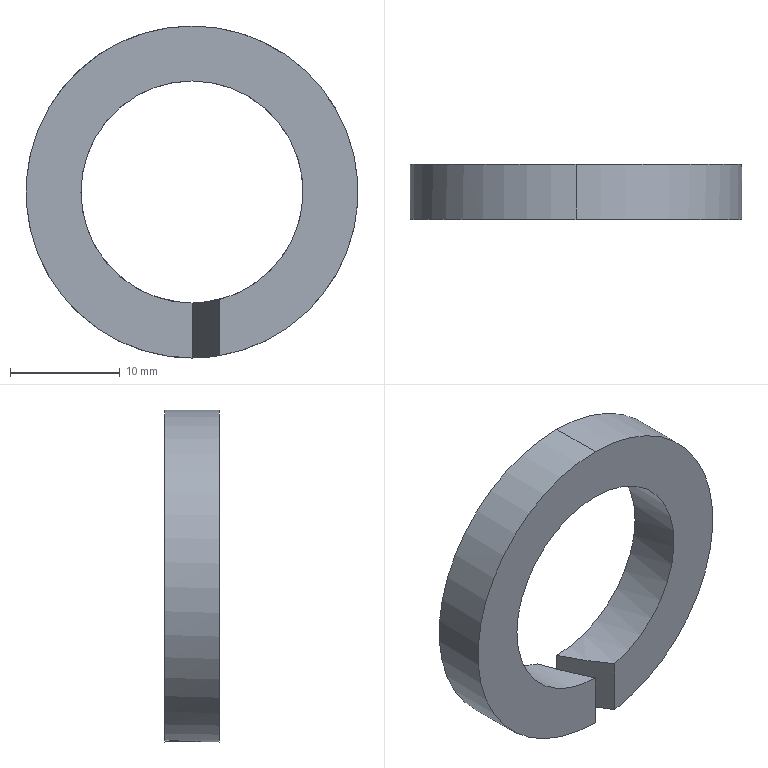Part | SolidWorks | features BaseBody 1 | 1 solid | 8 faces | box 30.2 x 5 x 30.2 mm | volume 1916 mm3 | cylinder 4 | plane 4 | commonest cylinder face diameters 20.2 x2 30.2 x2
STEP:
#1=CARTESIAN_POINT('',(2.5,0.,-9.786));
#2=VERTEX_POINT('',#1);
#3=CARTESIAN_POINT('',(0.,0.,10.1));
#4=VERTEX_POINT('',#3);
#5=CARTESIAN_POINT('',(0.,0.,0.));
#6=DIRECTION('',(0.,-1.,0.));
#7=DIRECTION('',(0.,0.,1.));
#8=AXIS2_PLACEMENT_3D('',#5,#6,#7);
#9=CIRCLE('',#8,10.1);
#10=EDGE_CURVE('',#2,#4,#9,.T.);
#11=ORIENTED_EDGE('',*,*,#10,.T.);
#12=CARTESIAN_POINT('',(0.,5.,10.1));
#13=VERTEX_POINT('',#12);
#14=CARTESIAN_POINT('',(0.,0.,10.1));
#15=DIRECTION('',(0.,1.,0.));
#16=VECTOR('',#15,1000.);
#17=LINE('',#14,#16);
#18=EDGE_CURVE('',#4,#13,#17,.T.);
#19=ORIENTED_EDGE('',*,*,#18,.T.);
#20=CARTESIAN_POINT('',(0.,5.,-10.1));
#21=VERTEX_POINT('',#20);
#22=CARTESIAN_POINT('',(0.,5.,0.));
#23=DIRECTION('',(0.,-1.,0.));
#24=DIRECTION('',(0.,0.,1.));
#25=AXIS2_PLACEMENT_3D('',#22,#23,#24);
#26=CIRCLE('',#25,10.1);
#27=EDGE_CURVE('',#21,#13,#26,.T.);
#28=ORIENTED_EDGE('',*,*,#27,.F.);
#29=CARTESIAN_POINT('',(2.5,0.,-9.786));
#30=CARTESIAN_POINT('',(1.682,1.636,-9.995));
#31=CARTESIAN_POINT('',(0.8443,3.311,-10.1));
#32=CARTESIAN_POINT('',(0.,5.,-10.1));
#33=(BOUNDED_CURVE()B_SPLINE_CURVE(3,(#29,#30,#31,#32),.UNSPECIFIED.,.F.,.F.)B_SPLINE_CURVE_WITH_KNOTS((4,4),(4.462,4.712),.UNSPECIFIED.)CURVE()GEOMETRIC_REPRESENTATION_ITEM()RATIONAL_B_SPLINE_CURVE((1.,0.9948,0.9948,1.))REPRESENTATION_ITEM(''));
#34=EDGE_CURVE('',#2,#21,#33,.T.);
#35=ORIENTED_EDGE('',*,*,#34,.F.);
#36=EDGE_LOOP('',(#11,#19,#28,#35));
#37=FACE_OUTER_BOUND('',#36,.T.);
#38=CARTESIAN_POINT('',(0.,0.,0.));
#39=DIRECTION('',(0.,1.,0.));
#40=DIRECTION('',(0.,0.,1.));
#41=AXIS2_PLACEMENT_3D('',#38,#39,#40);
#42=CYLINDRICAL_SURFACE('',#41,10.1);
#43=ADVANCED_FACE('',(#37),#42,.F.);
#44=CARTESIAN_POINT('',(0.,0.,-15.1));
#45=VERTEX_POINT('',#44);
#46=CARTESIAN_POINT('',(0.,0.,15.1));
#47=VERTEX_POINT('',#46);
#48=CARTESIAN_POINT('',(0.,0.,0.));
#49=DIRECTION('',(0.,1.,0.));
#50=DIRECTION('',(0.,0.,1.));
#51=AXIS2_PLACEMENT_3D('',#48,#49,#50);
#52=CIRCLE('',#51,15.1);
#53=EDGE_CURVE('',#45,#47,#52,.T.);
#54=ORIENTED_EDGE('',*,*,#53,.T.);
#55=CARTESIAN_POINT('',(0.,5.,15.1));
#56=VERTEX_POINT('',#55);
#57=CARTESIAN_POINT('',(0.,0.,15.1));
#58=DIRECTION('',(0.,1.,0.));
#59=VECTOR('',#58,1000.);
#60=LINE('',#57,#59);
#61=EDGE_CURVE('',#47,#56,#60,.T.);
#62=ORIENTED_EDGE('',*,*,#61,.T.);
#63=CARTESIAN_POINT('',(-2.5,5.,-14.892));
#64=VERTEX_POINT('',#63);
#65=CARTESIAN_POINT('',(0.,5.,0.));
#66=DIRECTION('',(0.,-1.,0.));
#67=DIRECTION('',(0.,0.,1.));
#68=AXIS2_PLACEMENT_3D('',#65,#66,#67);
#69=CIRCLE('',#68,15.1);
#70=EDGE_CURVE('',#56,#64,#69,.T.);
#71=ORIENTED_EDGE('',*,*,#70,.T.);
#72=CARTESIAN_POINT('',(-2.5,5.,-14.892));
#73=CARTESIAN_POINT('',(-1.673,3.347,-15.03));
#74=CARTESIAN_POINT('',(-0.8382,1.676,-15.1));
#75=CARTESIAN_POINT('',(0.,0.,-15.1));
#76=(BOUNDED_CURVE()B_SPLINE_CURVE(3,(#72,#73,#74,#75),.UNSPECIFIED.,.F.,.F.)B_SPLINE_CURVE_WITH_KNOTS((4,4),(1.404,1.571),.UNSPECIFIED.)CURVE()GEOMETRIC_REPRESENTATION_ITEM()RATIONAL_B_SPLINE_CURVE((1.,0.9977,0.9977,1.))REPRESENTATION_ITEM(''));
#77=EDGE_CURVE('',#64,#45,#76,.T.);
#78=ORIENTED_EDGE('',*,*,#77,.T.);
#79=EDGE_LOOP('',(#54,#62,#71,#78));
#80=FACE_OUTER_BOUND('',#79,.T.);
#81=CARTESIAN_POINT('',(0.,0.,0.));
#82=DIRECTION('',(0.,1.,0.));
#83=DIRECTION('',(0.,0.,1.));
#84=AXIS2_PLACEMENT_3D('',#81,#82,#83);
#85=CYLINDRICAL_SURFACE('',#84,15.1);
#86=ADVANCED_FACE('',(#80),#85,.T.);
#87=CARTESIAN_POINT('',(2.5,0.,-14.892));
#88=VERTEX_POINT('',#87);
#89=CARTESIAN_POINT('',(2.5,0.,0.));
#90=DIRECTION('',(0.,0.,1.));
#91=VECTOR('',#90,1000.);
#92=LINE('',#89,#91);
#93=EDGE_CURVE('',#88,#2,#92,.T.);
#94=ORIENTED_EDGE('',*,*,#93,.F.);
#95=CARTESIAN_POINT('',(0.,0.,0.));
#96=DIRECTION('',(0.,1.,0.));
#97=DIRECTION('',(0.,0.,1.));
#98=AXIS2_PLACEMENT_3D('',#95,#96,#97);
#99=CIRCLE('',#98,15.1);
#100=EDGE_CURVE('',#47,#88,#99,.T.);
#101=ORIENTED_EDGE('',*,*,#100,.F.);
#102=ORIENTED_EDGE('',*,*,#53,.F.);
#103=CARTESIAN_POINT('',(0.,0.,-10.1));
#104=VERTEX_POINT('',#103);
#105=CARTESIAN_POINT('',(0.,0.,0.));
#106=DIRECTION('',(0.,0.,-1.));
#107=VECTOR('',#106,1000.);
#108=LINE('',#105,#107);
#109=EDGE_CURVE('',#104,#45,#108,.T.);
#110=ORIENTED_EDGE('',*,*,#109,.F.);
#111=CARTESIAN_POINT('',(0.,0.,0.));
#112=DIRECTION('',(0.,-1.,0.));
#113=DIRECTION('',(0.,0.,1.));
#114=AXIS2_PLACEMENT_3D('',#111,#112,#113);
#115=CIRCLE('',#114,10.1);
#116=EDGE_CURVE('',#4,#104,#115,.T.);
#117=ORIENTED_EDGE('',*,*,#116,.F.);
#118=ORIENTED_EDGE('',*,*,#10,.F.);
#119=EDGE_LOOP('',(#94,#101,#102,#110,#117,#118));
#120=FACE_OUTER_BOUND('',#119,.T.);
#121=CARTESIAN_POINT('',(0.,0.,0.));
#122=DIRECTION('',(0.,1.,0.));
#123=DIRECTION('',(0.,0.,1.));
#124=AXIS2_PLACEMENT_3D('',#121,#122,#123);
#125=PLANE('',#124);
#126=ADVANCED_FACE('',(#120),#125,.F.);
#127=ORIENTED_EDGE('',*,*,#18,.F.);
#128=ORIENTED_EDGE('',*,*,#116,.T.);
#129=CARTESIAN_POINT('',(-2.5,5.,-9.786));
#130=VERTEX_POINT('',#129);
#131=CARTESIAN_POINT('',(0.,0.,-10.1));
#132=CARTESIAN_POINT('',(-0.8443,1.689,-10.1));
#133=CARTESIAN_POINT('',(-1.682,3.364,-9.995));
#134=CARTESIAN_POINT('',(-2.5,5.,-9.786));
#135=(BOUNDED_CURVE()B_SPLINE_CURVE(3,(#131,#132,#133,#134),.UNSPECIFIED.,.F.,.F.)B_SPLINE_CURVE_WITH_KNOTS((4,4),(4.712,4.963),.UNSPECIFIED.)CURVE()GEOMETRIC_REPRESENTATION_ITEM()RATIONAL_B_SPLINE_CURVE((1.,0.9948,0.9948,1.))REPRESENTATION_ITEM(''));
#136=EDGE_CURVE('',#104,#130,#135,.T.);
#137=ORIENTED_EDGE('',*,*,#136,.T.);
#138=CARTESIAN_POINT('',(0.,5.,0.));
#139=DIRECTION('',(0.,-1.,0.));
#140=DIRECTION('',(0.,0.,1.));
#141=AXIS2_PLACEMENT_3D('',#138,#139,#140);
#142=CIRCLE('',#141,10.1);
#143=EDGE_CURVE('',#13,#130,#142,.T.);
#144=ORIENTED_EDGE('',*,*,#143,.F.);
#145=EDGE_LOOP('',(#127,#128,#137,#144));
#146=FACE_OUTER_BOUND('',#145,.T.);
#147=CARTESIAN_POINT('',(0.,0.,0.));
#148=DIRECTION('',(0.,1.,0.));
#149=DIRECTION('',(0.,0.,1.));
#150=AXIS2_PLACEMENT_3D('',#147,#148,#149);
#151=CYLINDRICAL_SURFACE('',#150,10.1);
#152=ADVANCED_FACE('',(#146),#151,.F.);
#153=ORIENTED_EDGE('',*,*,#34,.T.);
#154=CARTESIAN_POINT('',(0.,5.,-15.1));
#155=VERTEX_POINT('',#154);
#156=CARTESIAN_POINT('',(0.,5.,0.));
#157=DIRECTION('',(0.,0.,1.));
#158=VECTOR('',#157,1000.);
#159=LINE('',#156,#158);
#160=EDGE_CURVE('',#155,#21,#159,.T.);
#161=ORIENTED_EDGE('',*,*,#160,.F.);
#162=CARTESIAN_POINT('',(2.5,0.,-14.892));
#163=CARTESIAN_POINT('',(1.673,1.653,-15.03));
#164=CARTESIAN_POINT('',(0.8382,3.324,-15.1));
#165=CARTESIAN_POINT('',(0.,5.,-15.1));
#166=(BOUNDED_CURVE()B_SPLINE_CURVE(3,(#162,#163,#164,#165),.UNSPECIFIED.,.F.,.T.)B_SPLINE_CURVE_WITH_KNOTS((4,4),(4.546,4.712),.UNSPECIFIED.)CURVE()GEOMETRIC_REPRESENTATION_ITEM()RATIONAL_B_SPLINE_CURVE((1.,0.9977,0.9977,1.))REPRESENTATION_ITEM(''));
#167=EDGE_CURVE('',#88,#155,#166,.T.);
#168=ORIENTED_EDGE('',*,*,#167,.F.);
#169=ORIENTED_EDGE('',*,*,#93,.T.);
#170=EDGE_LOOP('',(#153,#161,#168,#169));
#171=FACE_OUTER_BOUND('',#170,.T.);
#172=CARTESIAN_POINT('',(2.5,0.,0.));
#173=DIRECTION('',(0.8944,0.4472,0.));
#174=DIRECTION('',(-0.4472,0.8944,0.));
#175=AXIS2_PLACEMENT_3D('',#172,#173,#174);
#176=PLANE('',#175);
#177=ADVANCED_FACE('',(#171),#176,.F.);
#178=ORIENTED_EDGE('',*,*,#61,.F.);
#179=ORIENTED_EDGE('',*,*,#100,.T.);
#180=ORIENTED_EDGE('',*,*,#167,.T.);
#181=CARTESIAN_POINT('',(0.,5.,0.));
#182=DIRECTION('',(0.,-1.,0.));
#183=DIRECTION('',(0.,0.,1.));
#184=AXIS2_PLACEMENT_3D('',#181,#182,#183);
#185=CIRCLE('',#184,15.1);
#186=EDGE_CURVE('',#155,#56,#185,.T.);
#187=ORIENTED_EDGE('',*,*,#186,.T.);
#188=EDGE_LOOP('',(#178,#179,#180,#187));
#189=FACE_OUTER_BOUND('',#188,.T.);
#190=CARTESIAN_POINT('',(0.,0.,0.));
#191=DIRECTION('',(0.,1.,0.));
#192=DIRECTION('',(0.,0.,1.));
#193=AXIS2_PLACEMENT_3D('',#190,#191,#192);
#194=CYLINDRICAL_SURFACE('',#193,15.1);
#195=ADVANCED_FACE('',(#189),#194,.T.);
#196=ORIENTED_EDGE('',*,*,#77,.F.);
#197=CARTESIAN_POINT('',(-2.5,5.,0.));
#198=DIRECTION('',(0.,0.,-1.));
#199=VECTOR('',#198,1000.);
#200=LINE('',#197,#199);
#201=EDGE_CURVE('',#130,#64,#200,.T.);
#202=ORIENTED_EDGE('',*,*,#201,.F.);
#203=ORIENTED_EDGE('',*,*,#136,.F.);
#204=ORIENTED_EDGE('',*,*,#109,.T.);
#205=EDGE_LOOP('',(#196,#202,#203,#204));
#206=FACE_OUTER_BOUND('',#205,.T.);
#207=CARTESIAN_POINT('',(-2.5,5.,0.));
#208=DIRECTION('',(-0.8944,-0.4472,0.));
#209=DIRECTION('',(0.4472,-0.8944,0.));
#210=AXIS2_PLACEMENT_3D('',#207,#208,#209);
#211=PLANE('',#210);
#212=ADVANCED_FACE('',(#206),#211,.F.);
#213=ORIENTED_EDGE('',*,*,#27,.T.);
#214=ORIENTED_EDGE('',*,*,#143,.T.);
#215=ORIENTED_EDGE('',*,*,#201,.T.);
#216=ORIENTED_EDGE('',*,*,#70,.F.);
#217=ORIENTED_EDGE('',*,*,#186,.F.);
#218=ORIENTED_EDGE('',*,*,#160,.T.);
#219=EDGE_LOOP('',(#213,#214,#215,#216,#217,#218));
#220=FACE_OUTER_BOUND('',#219,.T.);
#221=CARTESIAN_POINT('',(0.,5.,0.));
#222=DIRECTION('',(0.,1.,0.));
#223=DIRECTION('',(0.,0.,1.));
#224=AXIS2_PLACEMENT_3D('',#221,#222,#223);
#225=PLANE('',#224);
#226=ADVANCED_FACE('',(#220),#225,.T.);
#227=CLOSED_SHELL('',(#43,#86,#126,#152,#177,#195,#212,#226));
#228=MANIFOLD_SOLID_BREP('',#227);
#229=CARTESIAN_POINT('',(0.,0.,0.));
#230=DIRECTION('',(0.,0.,1.));
#231=DIRECTION('',(1.,0.,0.));
#232=AXIS2_PLACEMENT_3D('',#229,#230,#231);
#233=(LENGTH_UNIT()NAMED_UNIT(*)SI_UNIT(.MILLI.,.METRE.));
#234=UNCERTAINTY_MEASURE_WITH_UNIT(LENGTH_MEASURE(0.00001),#233,'','');
#235=(NAMED_UNIT(*)PLANE_ANGLE_UNIT()SI_UNIT($,.RADIAN.));
#236=(NAMED_UNIT(*)SI_UNIT($,.STERADIAN.)SOLID_ANGLE_UNIT());
#237=(GEOMETRIC_REPRESENTATION_CONTEXT(3)GLOBAL_UNCERTAINTY_ASSIGNED_CONTEXT((#234))GLOBAL_UNIT_ASSIGNED_CONTEXT((#233,#235,#236))REPRESENTATION_CONTEXT('',''));
#238=ADVANCED_BREP_SHAPE_REPRESENTATION('',(#228,#232),#237);